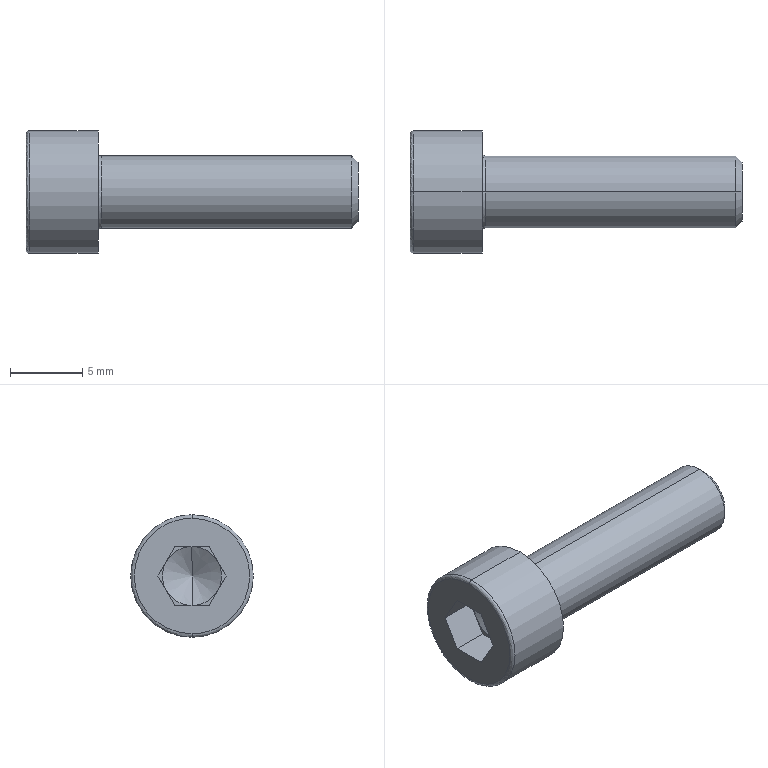Part | STEP file | 0243_305_SCB5-18 | 1 solid | 27 faces | box 23 x 8.5 x 8.5 mm | volume 594.23 mm3 | plane 15 | spline 4 | cylinder 4 | cone 4 | commonest cylinder face diameters 5 x2 8.5 x2